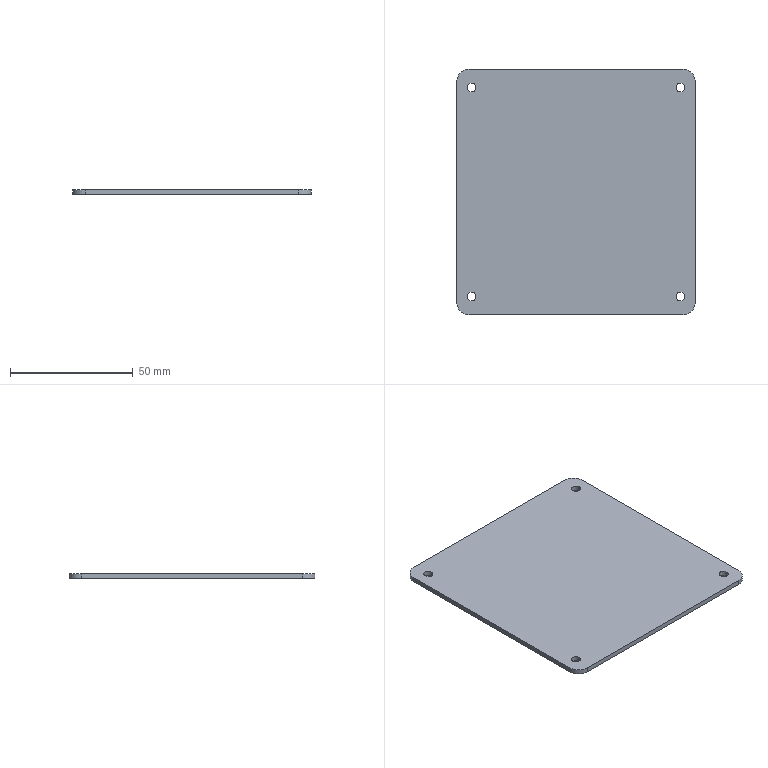Part | SolidWorks | features BaseBody 1 | 1 solid | 18 faces | box 97 x 100 x 2 mm | volume 19276 mm3 | cylinder 12 | plane 6 | commonest cylinder face diameters 3.6 x8 10 x4
STEP:
#1=CARTESIAN_POINT('',(44.3,42.5,2.));
#2=VERTEX_POINT('',#1);
#3=CARTESIAN_POINT('',(40.7,42.5,2.));
#4=VERTEX_POINT('',#3);
#5=CARTESIAN_POINT('',(42.5,42.5,2.));
#6=DIRECTION('',(0.,0.,-1.));
#7=DIRECTION('',(-1.,0.,0.));
#8=AXIS2_PLACEMENT_3D('',#5,#6,#7);
#9=CIRCLE('',#8,1.8);
#10=EDGE_CURVE('',#2,#4,#9,.T.);
#11=ORIENTED_EDGE('',*,*,#10,.F.);
#12=CARTESIAN_POINT('',(44.3,42.5,0.));
#13=VERTEX_POINT('',#12);
#14=CARTESIAN_POINT('',(44.3,42.5,0.));
#15=DIRECTION('',(0.,0.,-1.));
#16=VECTOR('',#15,1000.);
#17=LINE('',#14,#16);
#18=EDGE_CURVE('',#2,#13,#17,.T.);
#19=ORIENTED_EDGE('',*,*,#18,.T.);
#20=CARTESIAN_POINT('',(40.7,42.5,0.));
#21=VERTEX_POINT('',#20);
#22=CARTESIAN_POINT('',(42.5,42.5,0.));
#23=DIRECTION('',(0.,0.,1.));
#24=DIRECTION('',(-1.,0.,0.));
#25=AXIS2_PLACEMENT_3D('',#22,#23,#24);
#26=CIRCLE('',#25,1.8);
#27=EDGE_CURVE('',#21,#13,#26,.T.);
#28=ORIENTED_EDGE('',*,*,#27,.F.);
#29=CARTESIAN_POINT('',(40.7,42.5,0.));
#30=DIRECTION('',(0.,0.,-1.));
#31=VECTOR('',#30,1000.);
#32=LINE('',#29,#31);
#33=EDGE_CURVE('',#4,#21,#32,.T.);
#34=ORIENTED_EDGE('',*,*,#33,.F.);
#35=EDGE_LOOP('',(#11,#19,#28,#34));
#36=FACE_OUTER_BOUND('',#35,.T.);
#37=CARTESIAN_POINT('',(42.5,42.5,0.));
#38=DIRECTION('',(0.,0.,-1.));
#39=DIRECTION('',(-1.,0.,0.));
#40=AXIS2_PLACEMENT_3D('',#37,#38,#39);
#41=CYLINDRICAL_SURFACE('',#40,1.8);
#42=ADVANCED_FACE('',(#36),#41,.F.);
#43=CARTESIAN_POINT('',(44.3,-42.5,2.));
#44=VERTEX_POINT('',#43);
#45=CARTESIAN_POINT('',(40.7,-42.5,2.));
#46=VERTEX_POINT('',#45);
#47=CARTESIAN_POINT('',(42.5,-42.5,2.));
#48=DIRECTION('',(0.,0.,-1.));
#49=DIRECTION('',(-1.,0.,0.));
#50=AXIS2_PLACEMENT_3D('',#47,#48,#49);
#51=CIRCLE('',#50,1.8);
#52=EDGE_CURVE('',#44,#46,#51,.T.);
#53=ORIENTED_EDGE('',*,*,#52,.F.);
#54=CARTESIAN_POINT('',(44.3,-42.5,0.));
#55=VERTEX_POINT('',#54);
#56=CARTESIAN_POINT('',(44.3,-42.5,0.));
#57=DIRECTION('',(0.,0.,-1.));
#58=VECTOR('',#57,1000.);
#59=LINE('',#56,#58);
#60=EDGE_CURVE('',#44,#55,#59,.T.);
#61=ORIENTED_EDGE('',*,*,#60,.T.);
#62=CARTESIAN_POINT('',(40.7,-42.5,0.));
#63=VERTEX_POINT('',#62);
#64=CARTESIAN_POINT('',(42.5,-42.5,0.));
#65=DIRECTION('',(0.,0.,1.));
#66=DIRECTION('',(-1.,0.,0.));
#67=AXIS2_PLACEMENT_3D('',#64,#65,#66);
#68=CIRCLE('',#67,1.8);
#69=EDGE_CURVE('',#63,#55,#68,.T.);
#70=ORIENTED_EDGE('',*,*,#69,.F.);
#71=CARTESIAN_POINT('',(40.7,-42.5,0.));
#72=DIRECTION('',(0.,0.,-1.));
#73=VECTOR('',#72,1000.);
#74=LINE('',#71,#73);
#75=EDGE_CURVE('',#46,#63,#74,.T.);
#76=ORIENTED_EDGE('',*,*,#75,.F.);
#77=EDGE_LOOP('',(#53,#61,#70,#76));
#78=FACE_OUTER_BOUND('',#77,.T.);
#79=CARTESIAN_POINT('',(42.5,-42.5,0.));
#80=DIRECTION('',(0.,0.,-1.));
#81=DIRECTION('',(-1.,0.,0.));
#82=AXIS2_PLACEMENT_3D('',#79,#80,#81);
#83=CYLINDRICAL_SURFACE('',#82,1.8);
#84=ADVANCED_FACE('',(#78),#83,.F.);
#85=CARTESIAN_POINT('',(-40.7,42.5,2.));
#86=VERTEX_POINT('',#85);
#87=CARTESIAN_POINT('',(-44.3,42.5,2.));
#88=VERTEX_POINT('',#87);
#89=CARTESIAN_POINT('',(-42.5,42.5,2.));
#90=DIRECTION('',(0.,0.,-1.));
#91=DIRECTION('',(-1.,0.,0.));
#92=AXIS2_PLACEMENT_3D('',#89,#90,#91);
#93=CIRCLE('',#92,1.8);
#94=EDGE_CURVE('',#86,#88,#93,.T.);
#95=ORIENTED_EDGE('',*,*,#94,.F.);
#96=CARTESIAN_POINT('',(-40.7,42.5,0.));
#97=VERTEX_POINT('',#96);
#98=CARTESIAN_POINT('',(-40.7,42.5,0.));
#99=DIRECTION('',(0.,0.,-1.));
#100=VECTOR('',#99,1000.);
#101=LINE('',#98,#100);
#102=EDGE_CURVE('',#86,#97,#101,.T.);
#103=ORIENTED_EDGE('',*,*,#102,.T.);
#104=CARTESIAN_POINT('',(-44.3,42.5,0.));
#105=VERTEX_POINT('',#104);
#106=CARTESIAN_POINT('',(-42.5,42.5,0.));
#107=DIRECTION('',(0.,0.,1.));
#108=DIRECTION('',(-1.,0.,0.));
#109=AXIS2_PLACEMENT_3D('',#106,#107,#108);
#110=CIRCLE('',#109,1.8);
#111=EDGE_CURVE('',#105,#97,#110,.T.);
#112=ORIENTED_EDGE('',*,*,#111,.F.);
#113=CARTESIAN_POINT('',(-44.3,42.5,0.));
#114=DIRECTION('',(0.,0.,-1.));
#115=VECTOR('',#114,1000.);
#116=LINE('',#113,#115);
#117=EDGE_CURVE('',#88,#105,#116,.T.);
#118=ORIENTED_EDGE('',*,*,#117,.F.);
#119=EDGE_LOOP('',(#95,#103,#112,#118));
#120=FACE_OUTER_BOUND('',#119,.T.);
#121=CARTESIAN_POINT('',(-42.5,42.5,0.));
#122=DIRECTION('',(0.,0.,-1.));
#123=DIRECTION('',(-1.,0.,0.));
#124=AXIS2_PLACEMENT_3D('',#121,#122,#123);
#125=CYLINDRICAL_SURFACE('',#124,1.8);
#126=ADVANCED_FACE('',(#120),#125,.F.);
#127=CARTESIAN_POINT('',(-40.7,-42.5,2.));
#128=VERTEX_POINT('',#127);
#129=CARTESIAN_POINT('',(-44.3,-42.5,2.));
#130=VERTEX_POINT('',#129);
#131=CARTESIAN_POINT('',(-42.5,-42.5,2.));
#132=DIRECTION('',(0.,0.,-1.));
#133=DIRECTION('',(-1.,0.,0.));
#134=AXIS2_PLACEMENT_3D('',#131,#132,#133);
#135=CIRCLE('',#134,1.8);
#136=EDGE_CURVE('',#128,#130,#135,.T.);
#137=ORIENTED_EDGE('',*,*,#136,.F.);
#138=CARTESIAN_POINT('',(-40.7,-42.5,0.));
#139=VERTEX_POINT('',#138);
#140=CARTESIAN_POINT('',(-40.7,-42.5,0.));
#141=DIRECTION('',(0.,0.,-1.));
#142=VECTOR('',#141,1000.);
#143=LINE('',#140,#142);
#144=EDGE_CURVE('',#128,#139,#143,.T.);
#145=ORIENTED_EDGE('',*,*,#144,.T.);
#146=CARTESIAN_POINT('',(-44.3,-42.5,0.));
#147=VERTEX_POINT('',#146);
#148=CARTESIAN_POINT('',(-42.5,-42.5,0.));
#149=DIRECTION('',(0.,0.,1.));
#150=DIRECTION('',(-1.,0.,0.));
#151=AXIS2_PLACEMENT_3D('',#148,#149,#150);
#152=CIRCLE('',#151,1.8);
#153=EDGE_CURVE('',#147,#139,#152,.T.);
#154=ORIENTED_EDGE('',*,*,#153,.F.);
#155=CARTESIAN_POINT('',(-44.3,-42.5,0.));
#156=DIRECTION('',(0.,0.,-1.));
#157=VECTOR('',#156,1000.);
#158=LINE('',#155,#157);
#159=EDGE_CURVE('',#130,#147,#158,.T.);
#160=ORIENTED_EDGE('',*,*,#159,.F.);
#161=EDGE_LOOP('',(#137,#145,#154,#160));
#162=FACE_OUTER_BOUND('',#161,.T.);
#163=CARTESIAN_POINT('',(-42.5,-42.5,0.));
#164=DIRECTION('',(0.,0.,-1.));
#165=DIRECTION('',(-1.,0.,0.));
#166=AXIS2_PLACEMENT_3D('',#163,#164,#165);
#167=CYLINDRICAL_SURFACE('',#166,1.8);
#168=ADVANCED_FACE('',(#162),#167,.F.);
#169=CARTESIAN_POINT('',(-43.5,-50.,2.));
#170=VERTEX_POINT('',#169);
#171=CARTESIAN_POINT('',(43.5,-50.,2.));
#172=VERTEX_POINT('',#171);
#173=CARTESIAN_POINT('',(0.,-50.,2.));
#174=DIRECTION('',(1.,0.,0.));
#175=VECTOR('',#174,1000.);
#176=LINE('',#173,#175);
#177=EDGE_CURVE('',#170,#172,#176,.T.);
#178=ORIENTED_EDGE('',*,*,#177,.T.);
#179=CARTESIAN_POINT('',(48.5,-45.,2.));
#180=VERTEX_POINT('',#179);
#181=CARTESIAN_POINT('',(43.5,-45.,2.));
#182=DIRECTION('',(0.,0.,1.));
#183=DIRECTION('',(-1.,0.,0.));
#184=AXIS2_PLACEMENT_3D('',#181,#182,#183);
#185=CIRCLE('',#184,5.);
#186=EDGE_CURVE('',#172,#180,#185,.T.);
#187=ORIENTED_EDGE('',*,*,#186,.T.);
#188=CARTESIAN_POINT('',(48.5,45.,2.));
#189=VERTEX_POINT('',#188);
#190=CARTESIAN_POINT('',(48.5,0.,2.));
#191=DIRECTION('',(0.,1.,0.));
#192=VECTOR('',#191,1000.);
#193=LINE('',#190,#192);
#194=EDGE_CURVE('',#180,#189,#193,.T.);
#195=ORIENTED_EDGE('',*,*,#194,.T.);
#196=CARTESIAN_POINT('',(43.5,50.,2.));
#197=VERTEX_POINT('',#196);
#198=CARTESIAN_POINT('',(43.5,45.,2.));
#199=DIRECTION('',(0.,0.,1.));
#200=DIRECTION('',(-1.,0.,0.));
#201=AXIS2_PLACEMENT_3D('',#198,#199,#200);
#202=CIRCLE('',#201,5.);
#203=EDGE_CURVE('',#189,#197,#202,.T.);
#204=ORIENTED_EDGE('',*,*,#203,.T.);
#205=CARTESIAN_POINT('',(-43.5,50.,2.));
#206=VERTEX_POINT('',#205);
#207=CARTESIAN_POINT('',(0.,50.,2.));
#208=DIRECTION('',(-1.,0.,0.));
#209=VECTOR('',#208,1000.);
#210=LINE('',#207,#209);
#211=EDGE_CURVE('',#197,#206,#210,.T.);
#212=ORIENTED_EDGE('',*,*,#211,.T.);
#213=CARTESIAN_POINT('',(-48.5,45.,2.));
#214=VERTEX_POINT('',#213);
#215=CARTESIAN_POINT('',(-43.5,45.,2.));
#216=DIRECTION('',(0.,0.,1.));
#217=DIRECTION('',(-1.,0.,0.));
#218=AXIS2_PLACEMENT_3D('',#215,#216,#217);
#219=CIRCLE('',#218,5.);
#220=EDGE_CURVE('',#206,#214,#219,.T.);
#221=ORIENTED_EDGE('',*,*,#220,.T.);
#222=CARTESIAN_POINT('',(-48.5,-45.,2.));
#223=VERTEX_POINT('',#222);
#224=CARTESIAN_POINT('',(-48.5,0.,2.));
#225=DIRECTION('',(0.,-1.,0.));
#226=VECTOR('',#225,1000.);
#227=LINE('',#224,#226);
#228=EDGE_CURVE('',#214,#223,#227,.T.);
#229=ORIENTED_EDGE('',*,*,#228,.T.);
#230=CARTESIAN_POINT('',(-43.5,-45.,2.));
#231=DIRECTION('',(0.,0.,1.));
#232=DIRECTION('',(-1.,0.,0.));
#233=AXIS2_PLACEMENT_3D('',#230,#231,#232);
#234=CIRCLE('',#233,5.);
#235=EDGE_CURVE('',#223,#170,#234,.T.);
#236=ORIENTED_EDGE('',*,*,#235,.T.);
#237=EDGE_LOOP('',(#178,#187,#195,#204,#212,#221,#229,#236));
#238=FACE_OUTER_BOUND('',#237,.T.);
#239=CARTESIAN_POINT('',(42.5,42.5,2.));
#240=DIRECTION('',(0.,0.,-1.));
#241=DIRECTION('',(-1.,0.,0.));
#242=AXIS2_PLACEMENT_3D('',#239,#240,#241);
#243=CIRCLE('',#242,1.8);
#244=EDGE_CURVE('',#4,#2,#243,.T.);
#245=ORIENTED_EDGE('',*,*,#244,.T.);
#246=ORIENTED_EDGE('',*,*,#10,.T.);
#247=EDGE_LOOP('',(#245,#246));
#248=FACE_BOUND('',#247,.T.);
#249=CARTESIAN_POINT('',(42.5,-42.5,2.));
#250=DIRECTION('',(0.,0.,-1.));
#251=DIRECTION('',(-1.,0.,0.));
#252=AXIS2_PLACEMENT_3D('',#249,#250,#251);
#253=CIRCLE('',#252,1.8);
#254=EDGE_CURVE('',#46,#44,#253,.T.);
#255=ORIENTED_EDGE('',*,*,#254,.T.);
#256=ORIENTED_EDGE('',*,*,#52,.T.);
#257=EDGE_LOOP('',(#255,#256));
#258=FACE_BOUND('',#257,.T.);
#259=CARTESIAN_POINT('',(-42.5,42.5,2.));
#260=DIRECTION('',(0.,0.,-1.));
#261=DIRECTION('',(-1.,0.,0.));
#262=AXIS2_PLACEMENT_3D('',#259,#260,#261);
#263=CIRCLE('',#262,1.8);
#264=EDGE_CURVE('',#88,#86,#263,.T.);
#265=ORIENTED_EDGE('',*,*,#264,.T.);
#266=ORIENTED_EDGE('',*,*,#94,.T.);
#267=EDGE_LOOP('',(#265,#266));
#268=FACE_BOUND('',#267,.T.);
#269=CARTESIAN_POINT('',(-42.5,-42.5,2.));
#270=DIRECTION('',(0.,0.,-1.));
#271=DIRECTION('',(-1.,0.,0.));
#272=AXIS2_PLACEMENT_3D('',#269,#270,#271);
#273=CIRCLE('',#272,1.8);
#274=EDGE_CURVE('',#130,#128,#273,.T.);
#275=ORIENTED_EDGE('',*,*,#274,.T.);
#276=ORIENTED_EDGE('',*,*,#136,.T.);
#277=EDGE_LOOP('',(#275,#276));
#278=FACE_BOUND('',#277,.T.);
#279=CARTESIAN_POINT('',(0.,0.,2.));
#280=DIRECTION('',(0.,0.,1.));
#281=DIRECTION('',(1.,0.,0.));
#282=AXIS2_PLACEMENT_3D('',#279,#280,#281);
#283=PLANE('',#282);
#284=ADVANCED_FACE('',(#238,#248,#258,#268,#278),#283,.T.);
#285=CARTESIAN_POINT('',(43.5,-50.,0.));
#286=VERTEX_POINT('',#285);
#287=CARTESIAN_POINT('',(48.5,-45.,0.));
#288=VERTEX_POINT('',#287);
#289=CARTESIAN_POINT('',(43.5,-45.,0.));
#290=DIRECTION('',(0.,0.,1.));
#291=DIRECTION('',(-1.,0.,0.));
#292=AXIS2_PLACEMENT_3D('',#289,#290,#291);
#293=CIRCLE('',#292,5.);
#294=EDGE_CURVE('',#286,#288,#293,.T.);
#295=ORIENTED_EDGE('',*,*,#294,.T.);
#296=CARTESIAN_POINT('',(48.5,-45.,2.));
#297=DIRECTION('',(0.,0.,1.));
#298=VECTOR('',#297,1000.);
#299=LINE('',#296,#298);
#300=EDGE_CURVE('',#288,#180,#299,.T.);
#301=ORIENTED_EDGE('',*,*,#300,.T.);
#302=ORIENTED_EDGE('',*,*,#186,.F.);
#303=CARTESIAN_POINT('',(43.5,-50.,2.));
#304=DIRECTION('',(0.,0.,-1.));
#305=VECTOR('',#304,1000.);
#306=LINE('',#303,#305);
#307=EDGE_CURVE('',#172,#286,#306,.T.);
#308=ORIENTED_EDGE('',*,*,#307,.T.);
#309=EDGE_LOOP('',(#295,#301,#302,#308));
#310=FACE_OUTER_BOUND('',#309,.T.);
#311=CARTESIAN_POINT('',(43.5,-45.,2.));
#312=DIRECTION('',(0.,0.,-1.));
#313=DIRECTION('',(-1.,0.,0.));
#314=AXIS2_PLACEMENT_3D('',#311,#312,#313);
#315=CYLINDRICAL_SURFACE('',#314,5.);
#316=ADVANCED_FACE('',(#310),#315,.T.);
#317=ORIENTED_EDGE('',*,*,#307,.F.);
#318=ORIENTED_EDGE('',*,*,#177,.F.);
#319=CARTESIAN_POINT('',(-43.5,-50.,0.));
#320=VERTEX_POINT('',#319);
#321=CARTESIAN_POINT('',(-43.5,-50.,2.));
#322=DIRECTION('',(0.,0.,1.));
#323=VECTOR('',#322,1000.);
#324=LINE('',#321,#323);
#325=EDGE_CURVE('',#320,#170,#324,.T.);
#326=ORIENTED_EDGE('',*,*,#325,.F.);
#327=CARTESIAN_POINT('',(-48.5,-50.,0.));
#328=DIRECTION('',(-1.,0.,0.));
#329=VECTOR('',#328,1000.);
#330=LINE('',#327,#329);
#331=EDGE_CURVE('',#286,#320,#330,.T.);
#332=ORIENTED_EDGE('',*,*,#331,.F.);
#333=EDGE_LOOP('',(#317,#318,#326,#332));
#334=FACE_OUTER_BOUND('',#333,.T.);
#335=CARTESIAN_POINT('',(-48.5,-50.,2.));
#336=DIRECTION('',(0.,1.,0.));
#337=DIRECTION('',(0.,0.,1.));
#338=AXIS2_PLACEMENT_3D('',#335,#336,#337);
#339=PLANE('',#338);
#340=ADVANCED_FACE('',(#334),#339,.F.);
#341=CARTESIAN_POINT('',(-48.5,-45.,0.));
#342=VERTEX_POINT('',#341);
#343=CARTESIAN_POINT('',(-43.5,-45.,0.));
#344=DIRECTION('',(0.,0.,1.));
#345=DIRECTION('',(-1.,0.,0.));
#346=AXIS2_PLACEMENT_3D('',#343,#344,#345);
#347=CIRCLE('',#346,5.);
#348=EDGE_CURVE('',#342,#320,#347,.T.);
#349=ORIENTED_EDGE('',*,*,#348,.T.);
#350=ORIENTED_EDGE('',*,*,#325,.T.);
#351=ORIENTED_EDGE('',*,*,#235,.F.);
#352=CARTESIAN_POINT('',(-48.5,-45.,2.));
#353=DIRECTION('',(0.,0.,-1.));
#354=VECTOR('',#353,1000.);
#355=LINE('',#352,#354);
#356=EDGE_CURVE('',#223,#342,#355,.T.);
#357=ORIENTED_EDGE('',*,*,#356,.T.);
#358=EDGE_LOOP('',(#349,#350,#351,#357));
#359=FACE_OUTER_BOUND('',#358,.T.);
#360=CARTESIAN_POINT('',(-43.5,-45.,2.));
#361=DIRECTION('',(0.,0.,-1.));
#362=DIRECTION('',(-1.,0.,0.));
#363=AXIS2_PLACEMENT_3D('',#360,#361,#362);
#364=CYLINDRICAL_SURFACE('',#363,5.);
#365=ADVANCED_FACE('',(#359),#364,.T.);
#366=ORIENTED_EDGE('',*,*,#356,.F.);
#367=ORIENTED_EDGE('',*,*,#228,.F.);
#368=CARTESIAN_POINT('',(-48.5,45.,0.));
#369=VERTEX_POINT('',#368);
#370=CARTESIAN_POINT('',(-48.5,45.,2.));
#371=DIRECTION('',(0.,0.,1.));
#372=VECTOR('',#371,1000.);
#373=LINE('',#370,#372);
#374=EDGE_CURVE('',#369,#214,#373,.T.);
#375=ORIENTED_EDGE('',*,*,#374,.F.);
#376=CARTESIAN_POINT('',(-48.5,50.,0.));
#377=DIRECTION('',(0.,1.,0.));
#378=VECTOR('',#377,1000.);
#379=LINE('',#376,#378);
#380=EDGE_CURVE('',#342,#369,#379,.T.);
#381=ORIENTED_EDGE('',*,*,#380,.F.);
#382=EDGE_LOOP('',(#366,#367,#375,#381));
#383=FACE_OUTER_BOUND('',#382,.T.);
#384=CARTESIAN_POINT('',(-48.5,50.,2.));
#385=DIRECTION('',(1.,0.,0.));
#386=DIRECTION('',(0.,1.,0.));
#387=AXIS2_PLACEMENT_3D('',#384,#385,#386);
#388=PLANE('',#387);
#389=ADVANCED_FACE('',(#383),#388,.F.);
#390=CARTESIAN_POINT('',(-43.5,50.,0.));
#391=VERTEX_POINT('',#390);
#392=CARTESIAN_POINT('',(-43.5,45.,0.));
#393=DIRECTION('',(0.,0.,1.));
#394=DIRECTION('',(-1.,0.,0.));
#395=AXIS2_PLACEMENT_3D('',#392,#393,#394);
#396=CIRCLE('',#395,5.);
#397=EDGE_CURVE('',#391,#369,#396,.T.);
#398=ORIENTED_EDGE('',*,*,#397,.T.);
#399=ORIENTED_EDGE('',*,*,#374,.T.);
#400=ORIENTED_EDGE('',*,*,#220,.F.);
#401=CARTESIAN_POINT('',(-43.5,50.,2.));
#402=DIRECTION('',(0.,0.,-1.));
#403=VECTOR('',#402,1000.);
#404=LINE('',#401,#403);
#405=EDGE_CURVE('',#206,#391,#404,.T.);
#406=ORIENTED_EDGE('',*,*,#405,.T.);
#407=EDGE_LOOP('',(#398,#399,#400,#406));
#408=FACE_OUTER_BOUND('',#407,.T.);
#409=CARTESIAN_POINT('',(-43.5,45.,2.));
#410=DIRECTION('',(0.,0.,-1.));
#411=DIRECTION('',(-1.,0.,0.));
#412=AXIS2_PLACEMENT_3D('',#409,#410,#411);
#413=CYLINDRICAL_SURFACE('',#412,5.);
#414=ADVANCED_FACE('',(#408),#413,.T.);
#415=CARTESIAN_POINT('',(43.5,50.,0.));
#416=VERTEX_POINT('',#415);
#417=CARTESIAN_POINT('',(43.5,50.,2.));
#418=DIRECTION('',(0.,0.,1.));
#419=VECTOR('',#418,1000.);
#420=LINE('',#417,#419);
#421=EDGE_CURVE('',#416,#197,#420,.T.);
#422=ORIENTED_EDGE('',*,*,#421,.F.);
#423=CARTESIAN_POINT('',(-48.5,50.,0.));
#424=DIRECTION('',(1.,0.,0.));
#425=VECTOR('',#424,1000.);
#426=LINE('',#423,#425);
#427=EDGE_CURVE('',#391,#416,#426,.T.);
#428=ORIENTED_EDGE('',*,*,#427,.F.);
#429=ORIENTED_EDGE('',*,*,#405,.F.);
#430=ORIENTED_EDGE('',*,*,#211,.F.);
#431=EDGE_LOOP('',(#422,#428,#429,#430));
#432=FACE_OUTER_BOUND('',#431,.T.);
#433=CARTESIAN_POINT('',(-48.5,50.,2.));
#434=DIRECTION('',(0.,-1.,0.));
#435=DIRECTION('',(0.,0.,-1.));
#436=AXIS2_PLACEMENT_3D('',#433,#434,#435);
#437=PLANE('',#436);
#438=ADVANCED_FACE('',(#432),#437,.F.);
#439=CARTESIAN_POINT('',(48.5,45.,0.));
#440=VERTEX_POINT('',#439);
#441=CARTESIAN_POINT('',(43.5,45.,0.));
#442=DIRECTION('',(0.,0.,1.));
#443=DIRECTION('',(-1.,0.,0.));
#444=AXIS2_PLACEMENT_3D('',#441,#442,#443);
#445=CIRCLE('',#444,5.);
#446=EDGE_CURVE('',#440,#416,#445,.T.);
#447=ORIENTED_EDGE('',*,*,#446,.T.);
#448=ORIENTED_EDGE('',*,*,#421,.T.);
#449=ORIENTED_EDGE('',*,*,#203,.F.);
#450=CARTESIAN_POINT('',(48.5,45.,2.));
#451=DIRECTION('',(0.,0.,-1.));
#452=VECTOR('',#451,1000.);
#453=LINE('',#450,#452);
#454=EDGE_CURVE('',#189,#440,#453,.T.);
#455=ORIENTED_EDGE('',*,*,#454,.T.);
#456=EDGE_LOOP('',(#447,#448,#449,#455));
#457=FACE_OUTER_BOUND('',#456,.T.);
#458=CARTESIAN_POINT('',(43.5,45.,2.));
#459=DIRECTION('',(0.,0.,-1.));
#460=DIRECTION('',(-1.,0.,0.));
#461=AXIS2_PLACEMENT_3D('',#458,#459,#460);
#462=CYLINDRICAL_SURFACE('',#461,5.);
#463=ADVANCED_FACE('',(#457),#462,.T.);
#464=ORIENTED_EDGE('',*,*,#454,.F.);
#465=ORIENTED_EDGE('',*,*,#194,.F.);
#466=ORIENTED_EDGE('',*,*,#300,.F.);
#467=CARTESIAN_POINT('',(48.5,50.,0.));
#468=DIRECTION('',(0.,-1.,0.));
#469=VECTOR('',#468,1000.);
#470=LINE('',#467,#469);
#471=EDGE_CURVE('',#440,#288,#470,.T.);
#472=ORIENTED_EDGE('',*,*,#471,.F.);
#473=EDGE_LOOP('',(#464,#465,#466,#472));
#474=FACE_OUTER_BOUND('',#473,.T.);
#475=CARTESIAN_POINT('',(48.5,50.,2.));
#476=DIRECTION('',(-1.,0.,0.));
#477=DIRECTION('',(0.,-1.,0.));
#478=AXIS2_PLACEMENT_3D('',#475,#476,#477);
#479=PLANE('',#478);
#480=ADVANCED_FACE('',(#474),#479,.F.);
#481=ORIENTED_EDGE('',*,*,#18,.F.);
#482=ORIENTED_EDGE('',*,*,#244,.F.);
#483=ORIENTED_EDGE('',*,*,#33,.T.);
#484=CARTESIAN_POINT('',(42.5,42.5,0.));
#485=DIRECTION('',(0.,0.,1.));
#486=DIRECTION('',(-1.,0.,0.));
#487=AXIS2_PLACEMENT_3D('',#484,#485,#486);
#488=CIRCLE('',#487,1.8);
#489=EDGE_CURVE('',#13,#21,#488,.T.);
#490=ORIENTED_EDGE('',*,*,#489,.F.);
#491=EDGE_LOOP('',(#481,#482,#483,#490));
#492=FACE_OUTER_BOUND('',#491,.T.);
#493=CARTESIAN_POINT('',(42.5,42.5,0.));
#494=DIRECTION('',(0.,0.,-1.));
#495=DIRECTION('',(-1.,0.,0.));
#496=AXIS2_PLACEMENT_3D('',#493,#494,#495);
#497=CYLINDRICAL_SURFACE('',#496,1.8);
#498=ADVANCED_FACE('',(#492),#497,.F.);
#499=ORIENTED_EDGE('',*,*,#60,.F.);
#500=ORIENTED_EDGE('',*,*,#254,.F.);
#501=ORIENTED_EDGE('',*,*,#75,.T.);
#502=CARTESIAN_POINT('',(42.5,-42.5,0.));
#503=DIRECTION('',(0.,0.,1.));
#504=DIRECTION('',(-1.,0.,0.));
#505=AXIS2_PLACEMENT_3D('',#502,#503,#504);
#506=CIRCLE('',#505,1.8);
#507=EDGE_CURVE('',#55,#63,#506,.T.);
#508=ORIENTED_EDGE('',*,*,#507,.F.);
#509=EDGE_LOOP('',(#499,#500,#501,#508));
#510=FACE_OUTER_BOUND('',#509,.T.);
#511=CARTESIAN_POINT('',(42.5,-42.5,0.));
#512=DIRECTION('',(0.,0.,-1.));
#513=DIRECTION('',(-1.,0.,0.));
#514=AXIS2_PLACEMENT_3D('',#511,#512,#513);
#515=CYLINDRICAL_SURFACE('',#514,1.8);
#516=ADVANCED_FACE('',(#510),#515,.F.);
#517=ORIENTED_EDGE('',*,*,#102,.F.);
#518=ORIENTED_EDGE('',*,*,#264,.F.);
#519=ORIENTED_EDGE('',*,*,#117,.T.);
#520=CARTESIAN_POINT('',(-42.5,42.5,0.));
#521=DIRECTION('',(0.,0.,1.));
#522=DIRECTION('',(-1.,0.,0.));
#523=AXIS2_PLACEMENT_3D('',#520,#521,#522);
#524=CIRCLE('',#523,1.8);
#525=EDGE_CURVE('',#97,#105,#524,.T.);
#526=ORIENTED_EDGE('',*,*,#525,.F.);
#527=EDGE_LOOP('',(#517,#518,#519,#526));
#528=FACE_OUTER_BOUND('',#527,.T.);
#529=CARTESIAN_POINT('',(-42.5,42.5,0.));
#530=DIRECTION('',(0.,0.,-1.));
#531=DIRECTION('',(-1.,0.,0.));
#532=AXIS2_PLACEMENT_3D('',#529,#530,#531);
#533=CYLINDRICAL_SURFACE('',#532,1.8);
#534=ADVANCED_FACE('',(#528),#533,.F.);
#535=ORIENTED_EDGE('',*,*,#144,.F.);
#536=ORIENTED_EDGE('',*,*,#274,.F.);
#537=ORIENTED_EDGE('',*,*,#159,.T.);
#538=CARTESIAN_POINT('',(-42.5,-42.5,0.));
#539=DIRECTION('',(0.,0.,1.));
#540=DIRECTION('',(-1.,0.,0.));
#541=AXIS2_PLACEMENT_3D('',#538,#539,#540);
#542=CIRCLE('',#541,1.8);
#543=EDGE_CURVE('',#139,#147,#542,.T.);
#544=ORIENTED_EDGE('',*,*,#543,.F.);
#545=EDGE_LOOP('',(#535,#536,#537,#544));
#546=FACE_OUTER_BOUND('',#545,.T.);
#547=CARTESIAN_POINT('',(-42.5,-42.5,0.));
#548=DIRECTION('',(0.,0.,-1.));
#549=DIRECTION('',(-1.,0.,0.));
#550=AXIS2_PLACEMENT_3D('',#547,#548,#549);
#551=CYLINDRICAL_SURFACE('',#550,1.8);
#552=ADVANCED_FACE('',(#546),#551,.F.);
#553=ORIENTED_EDGE('',*,*,#446,.F.);
#554=ORIENTED_EDGE('',*,*,#471,.T.);
#555=ORIENTED_EDGE('',*,*,#294,.F.);
#556=ORIENTED_EDGE('',*,*,#331,.T.);
#557=ORIENTED_EDGE('',*,*,#348,.F.);
#558=ORIENTED_EDGE('',*,*,#380,.T.);
#559=ORIENTED_EDGE('',*,*,#397,.F.);
#560=ORIENTED_EDGE('',*,*,#427,.T.);
#561=EDGE_LOOP('',(#553,#554,#555,#556,#557,#558,#559,#560));
#562=FACE_OUTER_BOUND('',#561,.T.);
#563=ORIENTED_EDGE('',*,*,#27,.T.);
#564=ORIENTED_EDGE('',*,*,#489,.T.);
#565=EDGE_LOOP('',(#563,#564));
#566=FACE_BOUND('',#565,.T.);
#567=ORIENTED_EDGE('',*,*,#69,.T.);
#568=ORIENTED_EDGE('',*,*,#507,.T.);
#569=EDGE_LOOP('',(#567,#568));
#570=FACE_BOUND('',#569,.T.);
#571=ORIENTED_EDGE('',*,*,#111,.T.);
#572=ORIENTED_EDGE('',*,*,#525,.T.);
#573=EDGE_LOOP('',(#571,#572));
#574=FACE_BOUND('',#573,.T.);
#575=ORIENTED_EDGE('',*,*,#153,.T.);
#576=ORIENTED_EDGE('',*,*,#543,.T.);
#577=EDGE_LOOP('',(#575,#576));
#578=FACE_BOUND('',#577,.T.);
#579=CARTESIAN_POINT('',(0.,0.,0.));
#580=DIRECTION('',(0.,0.,1.));
#581=DIRECTION('',(1.,0.,0.));
#582=AXIS2_PLACEMENT_3D('',#579,#580,#581);
#583=PLANE('',#582);
#584=ADVANCED_FACE('',(#562,#566,#570,#574,#578),#583,.F.);
#585=CLOSED_SHELL('',(#42,#84,#126,#168,#284,#316,#340,#365,#389,#414,#438,#463,#480,#498,#516,#534,#552,#584));
#586=MANIFOLD_SOLID_BREP('',#585);
#587=CARTESIAN_POINT('',(0.,0.,0.));
#588=DIRECTION('',(0.,0.,1.));
#589=DIRECTION('',(1.,0.,0.));
#590=AXIS2_PLACEMENT_3D('',#587,#588,#589);
#591=(LENGTH_UNIT()NAMED_UNIT(*)SI_UNIT(.MILLI.,.METRE.));
#592=UNCERTAINTY_MEASURE_WITH_UNIT(LENGTH_MEASURE(0.00001),#591,'','');
#593=(NAMED_UNIT(*)PLANE_ANGLE_UNIT()SI_UNIT($,.RADIAN.));
#594=(NAMED_UNIT(*)SI_UNIT($,.STERADIAN.)SOLID_ANGLE_UNIT());
#595=(GEOMETRIC_REPRESENTATION_CONTEXT(3)GLOBAL_UNCERTAINTY_ASSIGNED_CONTEXT((#592))GLOBAL_UNIT_ASSIGNED_CONTEXT((#591,#593,#594))REPRESENTATION_CONTEXT('',''));
#596=ADVANCED_BREP_SHAPE_REPRESENTATION('',(#586,#590),#595);